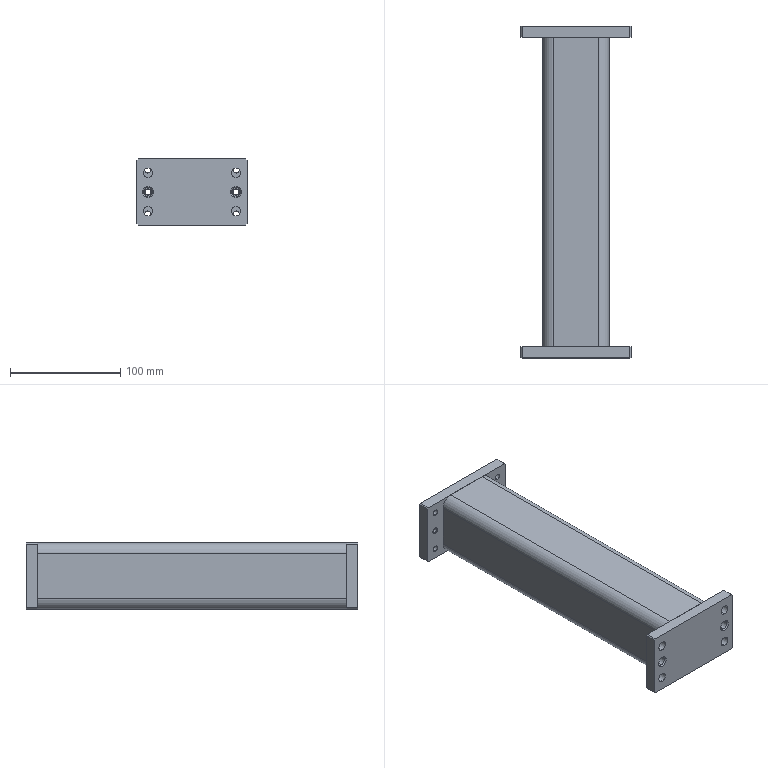Part | SolidWorks | features Chamfer 4, ICE 4, HoleWzd 2, 3DProfileFeature 1, WeldMemberFeat 1, WeldmentFeature 1 | 3 solids | 78 faces | box 100 x 301.5 x 60 mm | volume 406752 mm3 | cylinder 32 | plane 30 | cone 16 | commonest cylinder face diameters 5.5 x8 8.6 x8 5 x4 8 x4 10 x4 20 x4